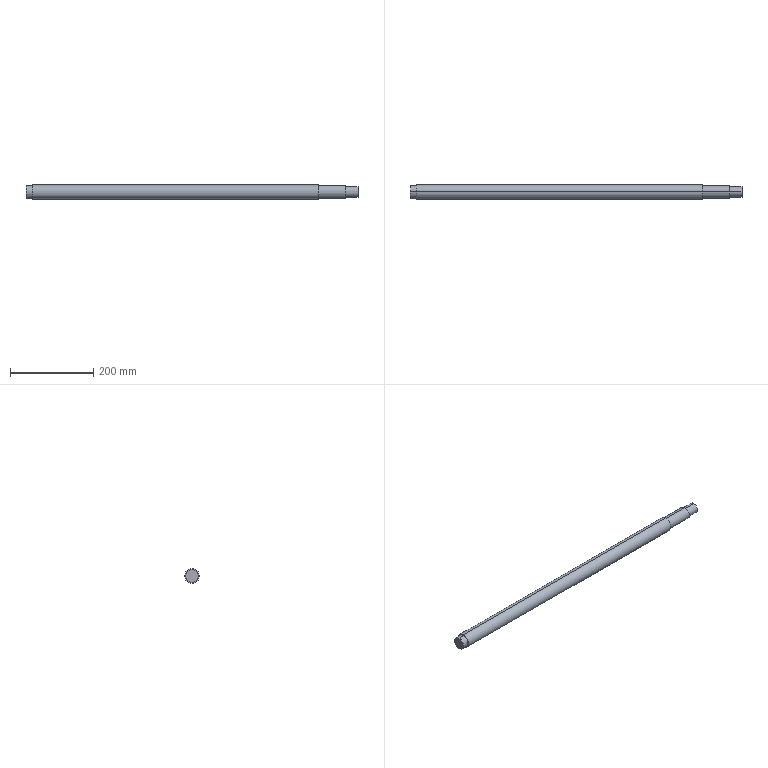Part | SolidWorks | features BaseBody 1 | 1 solid | 13 faces | box 796 x 35 x 35 mm | volume 731284 mm3 | cylinder 8 | plane 5 | commonest cylinder face diameters 30 x4 25 x2 35 x2
STEP:
#1=CARTESIAN_POINT('',(15.,0.,-17.5));
#2=VERTEX_POINT('',#1);
#3=CARTESIAN_POINT('',(15.,0.,17.5));
#4=VERTEX_POINT('',#3);
#5=CARTESIAN_POINT('',(15.,0.,0.));
#6=DIRECTION('',(1.,0.,0.));
#7=DIRECTION('',(0.,0.,-1.));
#8=AXIS2_PLACEMENT_3D('',#5,#6,#7);
#9=CIRCLE('',#8,17.5);
#10=EDGE_CURVE('',#2,#4,#9,.T.);
#11=ORIENTED_EDGE('',*,*,#10,.T.);
#12=CARTESIAN_POINT('',(701.,0.,17.5));
#13=VERTEX_POINT('',#12);
#14=CARTESIAN_POINT('',(0.,0.,17.5));
#15=DIRECTION('',(1.,0.,0.));
#16=VECTOR('',#15,1000.);
#17=LINE('',#14,#16);
#18=EDGE_CURVE('',#4,#13,#17,.T.);
#19=ORIENTED_EDGE('',*,*,#18,.T.);
#20=CARTESIAN_POINT('',(701.,0.,-17.5));
#21=VERTEX_POINT('',#20);
#22=CARTESIAN_POINT('',(701.,0.,0.));
#23=DIRECTION('',(-1.,0.,0.));
#24=DIRECTION('',(0.,0.,-1.));
#25=AXIS2_PLACEMENT_3D('',#22,#23,#24);
#26=CIRCLE('',#25,17.5);
#27=EDGE_CURVE('',#13,#21,#26,.T.);
#28=ORIENTED_EDGE('',*,*,#27,.T.);
#29=CARTESIAN_POINT('',(0.,0.,-17.5));
#30=DIRECTION('',(1.,0.,0.));
#31=VECTOR('',#30,1000.);
#32=LINE('',#29,#31);
#33=EDGE_CURVE('',#2,#21,#32,.T.);
#34=ORIENTED_EDGE('',*,*,#33,.F.);
#35=EDGE_LOOP('',(#11,#19,#28,#34));
#36=FACE_OUTER_BOUND('',#35,.T.);
#37=CARTESIAN_POINT('',(0.,0.,0.));
#38=DIRECTION('',(1.,0.,0.));
#39=DIRECTION('',(0.,0.,-1.));
#40=AXIS2_PLACEMENT_3D('',#37,#38,#39);
#41=CYLINDRICAL_SURFACE('',#40,17.5);
#42=ADVANCED_FACE('',(#36),#41,.T.);
#43=CARTESIAN_POINT('',(701.,0.,15.));
#44=VERTEX_POINT('',#43);
#45=CARTESIAN_POINT('',(701.,0.,-15.));
#46=VERTEX_POINT('',#45);
#47=CARTESIAN_POINT('',(701.,0.,0.));
#48=DIRECTION('',(-1.,0.,0.));
#49=DIRECTION('',(0.,0.,-1.));
#50=AXIS2_PLACEMENT_3D('',#47,#48,#49);
#51=CIRCLE('',#50,15.);
#52=EDGE_CURVE('',#44,#46,#51,.T.);
#53=ORIENTED_EDGE('',*,*,#52,.F.);
#54=CARTESIAN_POINT('',(766.,0.,15.));
#55=VERTEX_POINT('',#54);
#56=CARTESIAN_POINT('',(0.,0.,15.));
#57=DIRECTION('',(1.,0.,0.));
#58=VECTOR('',#57,1000.);
#59=LINE('',#56,#58);
#60=EDGE_CURVE('',#44,#55,#59,.T.);
#61=ORIENTED_EDGE('',*,*,#60,.T.);
#62=CARTESIAN_POINT('',(766.,0.,-15.));
#63=VERTEX_POINT('',#62);
#64=CARTESIAN_POINT('',(766.,0.,0.));
#65=DIRECTION('',(-1.,0.,0.));
#66=DIRECTION('',(0.,0.,-1.));
#67=AXIS2_PLACEMENT_3D('',#64,#65,#66);
#68=CIRCLE('',#67,15.);
#69=EDGE_CURVE('',#55,#63,#68,.T.);
#70=ORIENTED_EDGE('',*,*,#69,.T.);
#71=CARTESIAN_POINT('',(0.,0.,-15.));
#72=DIRECTION('',(1.,0.,0.));
#73=VECTOR('',#72,1000.);
#74=LINE('',#71,#73);
#75=EDGE_CURVE('',#46,#63,#74,.T.);
#76=ORIENTED_EDGE('',*,*,#75,.F.);
#77=EDGE_LOOP('',(#53,#61,#70,#76));
#78=FACE_OUTER_BOUND('',#77,.T.);
#79=CARTESIAN_POINT('',(0.,0.,0.));
#80=DIRECTION('',(1.,0.,0.));
#81=DIRECTION('',(0.,0.,-1.));
#82=AXIS2_PLACEMENT_3D('',#79,#80,#81);
#83=CYLINDRICAL_SURFACE('',#82,15.);
#84=ADVANCED_FACE('',(#78),#83,.T.);
#85=CARTESIAN_POINT('',(0.,0.,-15.));
#86=VERTEX_POINT('',#85);
#87=CARTESIAN_POINT('',(0.,0.,15.));
#88=VERTEX_POINT('',#87);
#89=CARTESIAN_POINT('',(0.,0.,0.));
#90=DIRECTION('',(1.,0.,0.));
#91=DIRECTION('',(0.,0.,-1.));
#92=AXIS2_PLACEMENT_3D('',#89,#90,#91);
#93=CIRCLE('',#92,15.);
#94=EDGE_CURVE('',#86,#88,#93,.T.);
#95=ORIENTED_EDGE('',*,*,#94,.T.);
#96=CARTESIAN_POINT('',(15.,0.,15.));
#97=VERTEX_POINT('',#96);
#98=CARTESIAN_POINT('',(0.,0.,15.));
#99=DIRECTION('',(1.,0.,0.));
#100=VECTOR('',#99,1000.);
#101=LINE('',#98,#100);
#102=EDGE_CURVE('',#88,#97,#101,.T.);
#103=ORIENTED_EDGE('',*,*,#102,.T.);
#104=CARTESIAN_POINT('',(15.,0.,-15.));
#105=VERTEX_POINT('',#104);
#106=CARTESIAN_POINT('',(15.,0.,0.));
#107=DIRECTION('',(1.,0.,0.));
#108=DIRECTION('',(0.,0.,-1.));
#109=AXIS2_PLACEMENT_3D('',#106,#107,#108);
#110=CIRCLE('',#109,15.);
#111=EDGE_CURVE('',#105,#97,#110,.T.);
#112=ORIENTED_EDGE('',*,*,#111,.F.);
#113=CARTESIAN_POINT('',(0.,0.,-15.));
#114=DIRECTION('',(1.,0.,0.));
#115=VECTOR('',#114,1000.);
#116=LINE('',#113,#115);
#117=EDGE_CURVE('',#86,#105,#116,.T.);
#118=ORIENTED_EDGE('',*,*,#117,.F.);
#119=EDGE_LOOP('',(#95,#103,#112,#118));
#120=FACE_OUTER_BOUND('',#119,.T.);
#121=CARTESIAN_POINT('',(0.,0.,0.));
#122=DIRECTION('',(1.,0.,0.));
#123=DIRECTION('',(0.,0.,-1.));
#124=AXIS2_PLACEMENT_3D('',#121,#122,#123);
#125=CYLINDRICAL_SURFACE('',#124,15.);
#126=ADVANCED_FACE('',(#120),#125,.T.);
#127=CARTESIAN_POINT('',(766.,0.,12.5));
#128=VERTEX_POINT('',#127);
#129=CARTESIAN_POINT('',(766.,0.,-12.5));
#130=VERTEX_POINT('',#129);
#131=CARTESIAN_POINT('',(766.,0.,0.));
#132=DIRECTION('',(-1.,0.,0.));
#133=DIRECTION('',(0.,0.,-1.));
#134=AXIS2_PLACEMENT_3D('',#131,#132,#133);
#135=CIRCLE('',#134,12.5);
#136=EDGE_CURVE('',#128,#130,#135,.T.);
#137=ORIENTED_EDGE('',*,*,#136,.F.);
#138=CARTESIAN_POINT('',(796.,0.,12.5));
#139=VERTEX_POINT('',#138);
#140=CARTESIAN_POINT('',(0.,0.,12.5));
#141=DIRECTION('',(1.,0.,0.));
#142=VECTOR('',#141,1000.);
#143=LINE('',#140,#142);
#144=EDGE_CURVE('',#128,#139,#143,.T.);
#145=ORIENTED_EDGE('',*,*,#144,.T.);
#146=CARTESIAN_POINT('',(796.,0.,-12.5));
#147=VERTEX_POINT('',#146);
#148=CARTESIAN_POINT('',(796.,0.,0.));
#149=DIRECTION('',(-1.,0.,0.));
#150=DIRECTION('',(0.,0.,-1.));
#151=AXIS2_PLACEMENT_3D('',#148,#149,#150);
#152=CIRCLE('',#151,12.5);
#153=EDGE_CURVE('',#139,#147,#152,.T.);
#154=ORIENTED_EDGE('',*,*,#153,.T.);
#155=CARTESIAN_POINT('',(0.,0.,-12.5));
#156=DIRECTION('',(1.,0.,0.));
#157=VECTOR('',#156,1000.);
#158=LINE('',#155,#157);
#159=EDGE_CURVE('',#130,#147,#158,.T.);
#160=ORIENTED_EDGE('',*,*,#159,.F.);
#161=EDGE_LOOP('',(#137,#145,#154,#160));
#162=FACE_OUTER_BOUND('',#161,.T.);
#163=CARTESIAN_POINT('',(0.,0.,0.));
#164=DIRECTION('',(1.,0.,0.));
#165=DIRECTION('',(0.,0.,-1.));
#166=AXIS2_PLACEMENT_3D('',#163,#164,#165);
#167=CYLINDRICAL_SURFACE('',#166,12.5);
#168=ADVANCED_FACE('',(#162),#167,.T.);
#169=ORIENTED_EDGE('',*,*,#18,.F.);
#170=CARTESIAN_POINT('',(15.,0.,0.));
#171=DIRECTION('',(1.,0.,0.));
#172=DIRECTION('',(0.,0.,-1.));
#173=AXIS2_PLACEMENT_3D('',#170,#171,#172);
#174=CIRCLE('',#173,17.5);
#175=EDGE_CURVE('',#4,#2,#174,.T.);
#176=ORIENTED_EDGE('',*,*,#175,.T.);
#177=ORIENTED_EDGE('',*,*,#33,.T.);
#178=CARTESIAN_POINT('',(701.,0.,0.));
#179=DIRECTION('',(-1.,0.,0.));
#180=DIRECTION('',(0.,0.,-1.));
#181=AXIS2_PLACEMENT_3D('',#178,#179,#180);
#182=CIRCLE('',#181,17.5);
#183=EDGE_CURVE('',#21,#13,#182,.T.);
#184=ORIENTED_EDGE('',*,*,#183,.T.);
#185=EDGE_LOOP('',(#169,#176,#177,#184));
#186=FACE_OUTER_BOUND('',#185,.T.);
#187=CARTESIAN_POINT('',(0.,0.,0.));
#188=DIRECTION('',(1.,0.,0.));
#189=DIRECTION('',(0.,0.,-1.));
#190=AXIS2_PLACEMENT_3D('',#187,#188,#189);
#191=CYLINDRICAL_SURFACE('',#190,17.5);
#192=ADVANCED_FACE('',(#186),#191,.T.);
#193=CARTESIAN_POINT('',(701.,0.,0.));
#194=DIRECTION('',(-1.,0.,0.));
#195=DIRECTION('',(0.,0.,-1.));
#196=AXIS2_PLACEMENT_3D('',#193,#194,#195);
#197=CIRCLE('',#196,15.);
#198=EDGE_CURVE('',#46,#44,#197,.T.);
#199=ORIENTED_EDGE('',*,*,#198,.T.);
#200=ORIENTED_EDGE('',*,*,#52,.T.);
#201=EDGE_LOOP('',(#199,#200));
#202=FACE_BOUND('',#201,.T.);
#203=ORIENTED_EDGE('',*,*,#183,.F.);
#204=ORIENTED_EDGE('',*,*,#27,.F.);
#205=EDGE_LOOP('',(#203,#204));
#206=FACE_OUTER_BOUND('',#205,.T.);
#207=CARTESIAN_POINT('',(701.,17.5,0.));
#208=DIRECTION('',(1.,0.,0.));
#209=DIRECTION('',(0.,0.,-1.));
#210=AXIS2_PLACEMENT_3D('',#207,#208,#209);
#211=PLANE('',#210);
#212=ADVANCED_FACE('',(#202,#206),#211,.T.);
#213=ORIENTED_EDGE('',*,*,#10,.F.);
#214=ORIENTED_EDGE('',*,*,#175,.F.);
#215=EDGE_LOOP('',(#213,#214));
#216=FACE_OUTER_BOUND('',#215,.T.);
#217=ORIENTED_EDGE('',*,*,#111,.T.);
#218=CARTESIAN_POINT('',(15.,0.,0.));
#219=DIRECTION('',(1.,0.,0.));
#220=DIRECTION('',(0.,0.,-1.));
#221=AXIS2_PLACEMENT_3D('',#218,#219,#220);
#222=CIRCLE('',#221,15.);
#223=EDGE_CURVE('',#97,#105,#222,.T.);
#224=ORIENTED_EDGE('',*,*,#223,.T.);
#225=EDGE_LOOP('',(#217,#224));
#226=FACE_BOUND('',#225,.T.);
#227=CARTESIAN_POINT('',(15.,15.,0.));
#228=DIRECTION('',(-1.,0.,0.));
#229=DIRECTION('',(0.,0.,1.));
#230=AXIS2_PLACEMENT_3D('',#227,#228,#229);
#231=PLANE('',#230);
#232=ADVANCED_FACE('',(#216,#226),#231,.T.);
#233=ORIENTED_EDGE('',*,*,#60,.F.);
#234=ORIENTED_EDGE('',*,*,#198,.F.);
#235=ORIENTED_EDGE('',*,*,#75,.T.);
#236=CARTESIAN_POINT('',(766.,0.,0.));
#237=DIRECTION('',(-1.,0.,0.));
#238=DIRECTION('',(0.,0.,-1.));
#239=AXIS2_PLACEMENT_3D('',#236,#237,#238);
#240=CIRCLE('',#239,15.);
#241=EDGE_CURVE('',#63,#55,#240,.T.);
#242=ORIENTED_EDGE('',*,*,#241,.T.);
#243=EDGE_LOOP('',(#233,#234,#235,#242));
#244=FACE_OUTER_BOUND('',#243,.T.);
#245=CARTESIAN_POINT('',(0.,0.,0.));
#246=DIRECTION('',(1.,0.,0.));
#247=DIRECTION('',(0.,0.,-1.));
#248=AXIS2_PLACEMENT_3D('',#245,#246,#247);
#249=CYLINDRICAL_SURFACE('',#248,15.);
#250=ADVANCED_FACE('',(#244),#249,.T.);
#251=ORIENTED_EDGE('',*,*,#102,.F.);
#252=CARTESIAN_POINT('',(0.,0.,0.));
#253=DIRECTION('',(1.,0.,0.));
#254=DIRECTION('',(0.,0.,-1.));
#255=AXIS2_PLACEMENT_3D('',#252,#253,#254);
#256=CIRCLE('',#255,15.);
#257=EDGE_CURVE('',#88,#86,#256,.T.);
#258=ORIENTED_EDGE('',*,*,#257,.T.);
#259=ORIENTED_EDGE('',*,*,#117,.T.);
#260=ORIENTED_EDGE('',*,*,#223,.F.);
#261=EDGE_LOOP('',(#251,#258,#259,#260));
#262=FACE_OUTER_BOUND('',#261,.T.);
#263=CARTESIAN_POINT('',(0.,0.,0.));
#264=DIRECTION('',(1.,0.,0.));
#265=DIRECTION('',(0.,0.,-1.));
#266=AXIS2_PLACEMENT_3D('',#263,#264,#265);
#267=CYLINDRICAL_SURFACE('',#266,15.);
#268=ADVANCED_FACE('',(#262),#267,.T.);
#269=CARTESIAN_POINT('',(766.,0.,0.));
#270=DIRECTION('',(-1.,0.,0.));
#271=DIRECTION('',(0.,0.,-1.));
#272=AXIS2_PLACEMENT_3D('',#269,#270,#271);
#273=CIRCLE('',#272,12.5);
#274=EDGE_CURVE('',#130,#128,#273,.T.);
#275=ORIENTED_EDGE('',*,*,#274,.T.);
#276=ORIENTED_EDGE('',*,*,#136,.T.);
#277=EDGE_LOOP('',(#275,#276));
#278=FACE_BOUND('',#277,.T.);
#279=ORIENTED_EDGE('',*,*,#241,.F.);
#280=ORIENTED_EDGE('',*,*,#69,.F.);
#281=EDGE_LOOP('',(#279,#280));
#282=FACE_OUTER_BOUND('',#281,.T.);
#283=CARTESIAN_POINT('',(766.,15.,0.));
#284=DIRECTION('',(1.,0.,0.));
#285=DIRECTION('',(0.,0.,-1.));
#286=AXIS2_PLACEMENT_3D('',#283,#284,#285);
#287=PLANE('',#286);
#288=ADVANCED_FACE('',(#278,#282),#287,.T.);
#289=ORIENTED_EDGE('',*,*,#94,.F.);
#290=ORIENTED_EDGE('',*,*,#257,.F.);
#291=EDGE_LOOP('',(#289,#290));
#292=FACE_OUTER_BOUND('',#291,.T.);
#293=CARTESIAN_POINT('',(0.,0.,0.));
#294=DIRECTION('',(-1.,0.,0.));
#295=DIRECTION('',(0.,0.,1.));
#296=AXIS2_PLACEMENT_3D('',#293,#294,#295);
#297=PLANE('',#296);
#298=ADVANCED_FACE('',(#292),#297,.T.);
#299=ORIENTED_EDGE('',*,*,#144,.F.);
#300=ORIENTED_EDGE('',*,*,#274,.F.);
#301=ORIENTED_EDGE('',*,*,#159,.T.);
#302=CARTESIAN_POINT('',(796.,0.,0.));
#303=DIRECTION('',(-1.,0.,0.));
#304=DIRECTION('',(0.,0.,-1.));
#305=AXIS2_PLACEMENT_3D('',#302,#303,#304);
#306=CIRCLE('',#305,12.5);
#307=EDGE_CURVE('',#147,#139,#306,.T.);
#308=ORIENTED_EDGE('',*,*,#307,.T.);
#309=EDGE_LOOP('',(#299,#300,#301,#308));
#310=FACE_OUTER_BOUND('',#309,.T.);
#311=CARTESIAN_POINT('',(0.,0.,0.));
#312=DIRECTION('',(1.,0.,0.));
#313=DIRECTION('',(0.,0.,-1.));
#314=AXIS2_PLACEMENT_3D('',#311,#312,#313);
#315=CYLINDRICAL_SURFACE('',#314,12.5);
#316=ADVANCED_FACE('',(#310),#315,.T.);
#317=ORIENTED_EDGE('',*,*,#307,.F.);
#318=ORIENTED_EDGE('',*,*,#153,.F.);
#319=EDGE_LOOP('',(#317,#318));
#320=FACE_OUTER_BOUND('',#319,.T.);
#321=CARTESIAN_POINT('',(796.,12.5,0.));
#322=DIRECTION('',(1.,0.,0.));
#323=DIRECTION('',(0.,0.,-1.));
#324=AXIS2_PLACEMENT_3D('',#321,#322,#323);
#325=PLANE('',#324);
#326=ADVANCED_FACE('',(#320),#325,.T.);
#327=CLOSED_SHELL('',(#42,#84,#126,#168,#192,#212,#232,#250,#268,#288,#298,#316,#326));
#328=MANIFOLD_SOLID_BREP('',#327);
#329=CARTESIAN_POINT('',(0.,0.,0.));
#330=DIRECTION('',(0.,0.,1.));
#331=DIRECTION('',(1.,0.,0.));
#332=AXIS2_PLACEMENT_3D('',#329,#330,#331);
#333=(LENGTH_UNIT()NAMED_UNIT(*)SI_UNIT(.MILLI.,.METRE.));
#334=UNCERTAINTY_MEASURE_WITH_UNIT(LENGTH_MEASURE(0.00001),#333,'','');
#335=(NAMED_UNIT(*)PLANE_ANGLE_UNIT()SI_UNIT($,.RADIAN.));
#336=(NAMED_UNIT(*)SI_UNIT($,.STERADIAN.)SOLID_ANGLE_UNIT());
#337=(GEOMETRIC_REPRESENTATION_CONTEXT(3)GLOBAL_UNCERTAINTY_ASSIGNED_CONTEXT((#334))GLOBAL_UNIT_ASSIGNED_CONTEXT((#333,#335,#336))REPRESENTATION_CONTEXT('',''));
#338=ADVANCED_BREP_SHAPE_REPRESENTATION('',(#328,#332),#337);